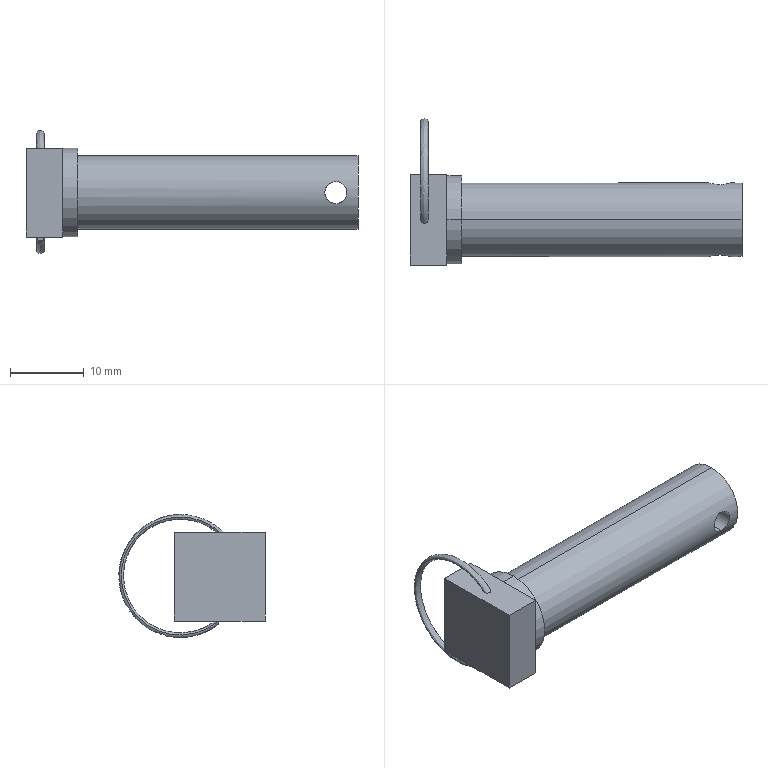Part | SolidWorks | features ICE 3, BaseBody 1, Sweep 1 | 1 solid | 20 faces | box 45 x 19.844 x 16.686 mm | volume 3901 mm3 | plane 10 | cylinder 8 | spline 2 | commonest cylinder face diameters 0.2 x2 3 x2 10 x2 12 x2
STEP:
#1=CARTESIAN_POINT('',(-3.551,0.1842,-6.026));
#2=VERTEX_POINT('',#1);
#3=CARTESIAN_POINT('',(-2.551,0.1842,-6.026));
#4=VERTEX_POINT('',#3);
#5=CARTESIAN_POINT('',(-3.051,0.1842,-6.026));
#6=DIRECTION('',(0.,-0.9908,-0.1352));
#7=DIRECTION('',(1.,0.,0.));
#8=AXIS2_PLACEMENT_3D('',#5,#6,#7);
#9=CIRCLE('',#8,0.5);
#10=EDGE_CURVE('',#2,#4,#9,.T.);
#11=ORIENTED_EDGE('',*,*,#10,.F.);
#12=CARTESIAN_POINT('',(-3.551,0.,6.026));
#13=VERTEX_POINT('',#12);
#14=CARTESIAN_POINT('',(-3.551,0.1842,-6.026));
#15=CARTESIAN_POINT('',(-3.551,6.268,-11.175));
#16=CARTESIAN_POINT('',(-3.551,13.473,-7.767));
#17=CARTESIAN_POINT('',(-3.551,13.351,0.2026));
#18=CARTESIAN_POINT('',(-3.551,13.229,8.172));
#19=CARTESIAN_POINT('',(-3.551,5.924,11.358));
#20=CARTESIAN_POINT('',(-3.551,0.,6.026));
#21=(BOUNDED_CURVE()B_SPLINE_CURVE(3,(#14,#15,#16,#17,#18,#19,#20),.UNSPECIFIED.,.F.,.F.)B_SPLINE_CURVE_WITH_KNOTS((4,3,4),(0.,0.5,1.),.UNSPECIFIED.)CURVE()GEOMETRIC_REPRESENTATION_ITEM()RATIONAL_B_SPLINE_CURVE((1.,0.6092,0.6092,1.,0.6092,0.6092,1.))REPRESENTATION_ITEM(''));
#22=EDGE_CURVE('',#2,#13,#21,.T.);
#23=ORIENTED_EDGE('',*,*,#22,.T.);
#24=CARTESIAN_POINT('',(-2.551,0.,6.026));
#25=VERTEX_POINT('',#24);
#26=CARTESIAN_POINT('',(-3.051,0.,6.026));
#27=DIRECTION('',(0.,0.,1.));
#28=DIRECTION('',(1.,0.,0.));
#29=AXIS2_PLACEMENT_3D('',#26,#27,#28);
#30=CIRCLE('',#29,0.5);
#31=EDGE_CURVE('',#13,#25,#30,.T.);
#32=ORIENTED_EDGE('',*,*,#31,.T.);
#33=CARTESIAN_POINT('',(-2.551,0.1842,-6.026));
#34=CARTESIAN_POINT('',(-2.551,6.268,-11.175));
#35=CARTESIAN_POINT('',(-2.551,13.473,-7.767));
#36=CARTESIAN_POINT('',(-2.551,13.351,0.2026));
#37=CARTESIAN_POINT('',(-2.551,13.229,8.172));
#38=CARTESIAN_POINT('',(-2.551,5.924,11.358));
#39=CARTESIAN_POINT('',(-2.551,0.,6.026));
#40=(BOUNDED_CURVE()B_SPLINE_CURVE(3,(#33,#34,#35,#36,#37,#38,#39),.UNSPECIFIED.,.F.,.T.)B_SPLINE_CURVE_WITH_KNOTS((4,3,4),(0.,0.5,1.),.UNSPECIFIED.)CURVE()GEOMETRIC_REPRESENTATION_ITEM()RATIONAL_B_SPLINE_CURVE((1.,0.6092,0.6092,1.,0.6092,0.6092,1.))REPRESENTATION_ITEM(''));
#41=EDGE_CURVE('',#4,#25,#40,.T.);
#42=ORIENTED_EDGE('',*,*,#41,.F.);
#43=EDGE_LOOP('',(#11,#23,#32,#42));
#44=FACE_OUTER_BOUND('',#43,.T.);
#45=CARTESIAN_POINT('',(-2.551,0.1842,-6.026));
#46=CARTESIAN_POINT('',(-2.551,6.268,-11.175));
#47=CARTESIAN_POINT('',(-2.551,13.473,-7.767));
#48=CARTESIAN_POINT('',(-2.551,13.351,0.2026));
#49=CARTESIAN_POINT('',(-2.551,13.229,8.172));
#50=CARTESIAN_POINT('',(-2.551,5.924,11.358));
#51=CARTESIAN_POINT('',(-2.551,0.,6.026));
#52=CARTESIAN_POINT('',(-2.551,0.04897,-5.036));
#53=CARTESIAN_POINT('',(-2.551,5.146,-10.319));
#54=CARTESIAN_POINT('',(-2.551,12.065,-7.865));
#55=CARTESIAN_POINT('',(-2.551,12.693,-0.5508));
#56=CARTESIAN_POINT('',(-2.551,13.322,6.763));
#57=CARTESIAN_POINT('',(-2.551,6.924,10.362));
#58=CARTESIAN_POINT('',(-2.551,1.,6.026));
#59=CARTESIAN_POINT('',(-3.551,0.04897,-5.036));
#60=CARTESIAN_POINT('',(-3.551,5.146,-10.319));
#61=CARTESIAN_POINT('',(-3.551,12.065,-7.865));
#62=CARTESIAN_POINT('',(-3.551,12.693,-0.5508));
#63=CARTESIAN_POINT('',(-3.551,13.322,6.763));
#64=CARTESIAN_POINT('',(-3.551,6.924,10.362));
#65=CARTESIAN_POINT('',(-3.551,1.,6.026));
#66=CARTESIAN_POINT('',(-3.551,0.1842,-6.026));
#67=CARTESIAN_POINT('',(-3.551,6.268,-11.175));
#68=CARTESIAN_POINT('',(-3.551,13.473,-7.767));
#69=CARTESIAN_POINT('',(-3.551,13.351,0.2026));
#70=CARTESIAN_POINT('',(-3.551,13.229,8.172));
#71=CARTESIAN_POINT('',(-3.551,5.924,11.358));
#72=CARTESIAN_POINT('',(-3.551,0.,6.026));
#73=CARTESIAN_POINT('',(-3.551,0.3194,-7.017));
#74=CARTESIAN_POINT('',(-3.551,7.391,-12.031));
#75=CARTESIAN_POINT('',(-3.551,14.881,-7.668));
#76=CARTESIAN_POINT('',(-3.551,14.009,0.956));
#77=CARTESIAN_POINT('',(-3.551,13.136,9.58));
#78=CARTESIAN_POINT('',(-3.551,4.924,12.355));
#79=CARTESIAN_POINT('',(-3.551,-1.,6.026));
#80=CARTESIAN_POINT('',(-2.551,0.3194,-7.017));
#81=CARTESIAN_POINT('',(-2.551,7.391,-12.031));
#82=CARTESIAN_POINT('',(-2.551,14.881,-7.668));
#83=CARTESIAN_POINT('',(-2.551,14.009,0.956));
#84=CARTESIAN_POINT('',(-2.551,13.136,9.58));
#85=CARTESIAN_POINT('',(-2.551,4.924,12.355));
#86=CARTESIAN_POINT('',(-2.551,-1.,6.026));
#87=CARTESIAN_POINT('',(-2.551,0.1842,-6.026));
#88=CARTESIAN_POINT('',(-2.551,6.268,-11.175));
#89=CARTESIAN_POINT('',(-2.551,13.473,-7.767));
#90=CARTESIAN_POINT('',(-2.551,13.351,0.2026));
#91=CARTESIAN_POINT('',(-2.551,13.229,8.172));
#92=CARTESIAN_POINT('',(-2.551,5.924,11.358));
#93=CARTESIAN_POINT('',(-2.551,0.,6.026));
#94=(BOUNDED_SURFACE()B_SPLINE_SURFACE(3,3,((#45,#46,#47,#48,#49,#50,#51),(#52,#53,#54,#55,#56,#57,#58),(#59,#60,#61,#62,#63,#64,#65),(#66,#67,#68,#69,#70,#71,#72),(#73,#74,#75,#76,#77,#78,#79),(#80,#81,#82,#83,#84,#85,#86),(#87,#88,#89,#90,#91,#92,#93)),.UNSPECIFIED.,.T.,.F.,.F.)B_SPLINE_SURFACE_WITH_KNOTS((4,3,4),(4,3,4),(0.,0.5,1.),(0.,0.5,1.),.UNSPECIFIED.)GEOMETRIC_REPRESENTATION_ITEM()RATIONAL_B_SPLINE_SURFACE(((1.,0.6092,0.6092,1.,0.6092,0.6092,1.),(0.3333,0.2031,0.2031,0.3333,0.2031,0.2031,0.3333),(0.3333,0.2031,0.2031,0.3333,0.2031,0.2031,0.3333),(1.,0.6092,0.6092,1.,0.6092,0.6092,1.),(0.3333,0.2031,0.2031,0.3333,0.2031,0.2031,0.3333),(0.3333,0.2031,0.2031,0.3333,0.2031,0.2031,0.3333),(1.,0.6092,0.6092,1.,0.6092,0.6092,1.)))REPRESENTATION_ITEM('')SURFACE());
#95=ADVANCED_FACE('',(#44),#94,.F.);
#96=CARTESIAN_POINT('',(-3.151,0.,-6.026));
#97=VERTEX_POINT('',#96);
#98=CARTESIAN_POINT('',(-2.951,0.,-6.026));
#99=VERTEX_POINT('',#98);
#100=CARTESIAN_POINT('',(-3.051,0.,-6.026));
#101=DIRECTION('',(0.,0.,1.));
#102=DIRECTION('',(1.,0.,0.));
#103=AXIS2_PLACEMENT_3D('',#100,#101,#102);
#104=CIRCLE('',#103,0.1);
#105=EDGE_CURVE('',#97,#99,#104,.T.);
#106=ORIENTED_EDGE('',*,*,#105,.F.);
#107=CARTESIAN_POINT('',(-3.151,0.,6.026));
#108=VERTEX_POINT('',#107);
#109=CARTESIAN_POINT('',(-3.151,0.,-6.026));
#110=DIRECTION('',(0.,0.,1.));
#111=VECTOR('',#110,1000.);
#112=LINE('',#109,#111);
#113=EDGE_CURVE('',#97,#108,#112,.T.);
#114=ORIENTED_EDGE('',*,*,#113,.T.);
#115=CARTESIAN_POINT('',(-2.951,0.,6.026));
#116=VERTEX_POINT('',#115);
#117=CARTESIAN_POINT('',(-3.051,0.,6.026));
#118=DIRECTION('',(0.,0.,1.));
#119=DIRECTION('',(1.,0.,0.));
#120=AXIS2_PLACEMENT_3D('',#117,#118,#119);
#121=CIRCLE('',#120,0.1);
#122=EDGE_CURVE('',#108,#116,#121,.T.);
#123=ORIENTED_EDGE('',*,*,#122,.T.);
#124=CARTESIAN_POINT('',(-2.951,0.,-6.026));
#125=DIRECTION('',(0.,0.,1.));
#126=VECTOR('',#125,1000.);
#127=LINE('',#124,#126);
#128=EDGE_CURVE('',#99,#116,#127,.T.);
#129=ORIENTED_EDGE('',*,*,#128,.F.);
#130=EDGE_LOOP('',(#106,#114,#123,#129));
#131=FACE_OUTER_BOUND('',#130,.T.);
#132=CARTESIAN_POINT('',(-3.051,0.,-6.026));
#133=DIRECTION('',(0.,0.,1.));
#134=DIRECTION('',(1.,0.,0.));
#135=AXIS2_PLACEMENT_3D('',#132,#133,#134);
#136=CYLINDRICAL_SURFACE('',#135,0.1);
#137=ADVANCED_FACE('',(#131),#136,.F.);
#138=CARTESIAN_POINT('',(37.,4.77,1.5));
#139=VERTEX_POINT('',#138);
#140=CARTESIAN_POINT('',(37.,4.77,-1.5));
#141=VERTEX_POINT('',#140);
#142=CARTESIAN_POINT('',(37.,4.77,1.5));
#143=CARTESIAN_POINT('',(36.9,4.77,1.5));
#144=CARTESIAN_POINT('',(36.802,4.773,1.49));
#145=CARTESIAN_POINT('',(36.61,4.785,1.452));
#146=CARTESIAN_POINT('',(36.514,4.794,1.423));
#147=CARTESIAN_POINT('',(36.333,4.815,1.347));
#148=CARTESIAN_POINT('',(36.247,4.828,1.301));
#149=CARTESIAN_POINT('',(36.085,4.856,1.192));
#150=CARTESIAN_POINT('',(36.008,4.871,1.129));
#151=CARTESIAN_POINT('',(35.802,4.916,0.9233));
#152=CARTESIAN_POINT('',(35.69,4.946,0.7569));
#153=CARTESIAN_POINT('',(35.54,4.988,0.3965));
#154=CARTESIAN_POINT('',(35.5,5.,0.1984));
#155=CARTESIAN_POINT('',(35.5,5.,-0.09698));
#156=CARTESIAN_POINT('',(35.51,4.997,-0.197));
#157=CARTESIAN_POINT('',(35.548,4.986,-0.3898));
#158=CARTESIAN_POINT('',(35.577,4.977,-0.4837));
#159=CARTESIAN_POINT('',(35.69,4.946,-0.7572));
#160=CARTESIAN_POINT('',(35.801,4.916,-0.9219));
#161=CARTESIAN_POINT('',(36.008,4.871,-1.13));
#162=CARTESIAN_POINT('',(36.083,4.856,-1.191));
#163=CARTESIAN_POINT('',(36.245,4.828,-1.3));
#164=CARTESIAN_POINT('',(36.333,4.815,-1.347));
#165=CARTESIAN_POINT('',(36.604,4.783,-1.46));
#166=CARTESIAN_POINT('',(36.801,4.77,-1.5));
#167=CARTESIAN_POINT('',(37.,4.77,-1.5));
#168=B_SPLINE_CURVE_WITH_KNOTS('',3,(#142,#143,#144,#145,#146,#147,#148,#149,#150,#151,#152,#153,#154,#155,#156,#157,#158,#159,#160,#161,#162,#163,#164,#165,#166,#167),.UNSPECIFIED.,.F.,.F.,(4,2,2,2,2,2,2,2,2,2,2,2,4),(0.004715,0.00501,0.005305,0.005599,0.005894,0.006483,0.007073,0.007367,0.007662,0.008251,0.008546,0.008841,0.00943),.UNSPECIFIED.);
#169=EDGE_CURVE('',#139,#141,#168,.T.);
#170=ORIENTED_EDGE('',*,*,#169,.T.);
#171=CARTESIAN_POINT('',(37.,4.77,-1.5));
#172=CARTESIAN_POINT('',(37.1,4.77,-1.5));
#173=CARTESIAN_POINT('',(37.198,4.773,-1.49));
#174=CARTESIAN_POINT('',(37.39,4.785,-1.452));
#175=CARTESIAN_POINT('',(37.486,4.794,-1.423));
#176=CARTESIAN_POINT('',(37.667,4.815,-1.347));
#177=CARTESIAN_POINT('',(37.753,4.828,-1.301));
#178=CARTESIAN_POINT('',(37.915,4.856,-1.192));
#179=CARTESIAN_POINT('',(37.992,4.871,-1.129));
#180=CARTESIAN_POINT('',(38.198,4.916,-0.9233));
#181=CARTESIAN_POINT('',(38.31,4.946,-0.7569));
#182=CARTESIAN_POINT('',(38.46,4.988,-0.3965));
#183=CARTESIAN_POINT('',(38.5,5.,-0.1984));
#184=CARTESIAN_POINT('',(38.5,5.,0.09698));
#185=CARTESIAN_POINT('',(38.49,4.997,0.197));
#186=CARTESIAN_POINT('',(38.452,4.986,0.3898));
#187=CARTESIAN_POINT('',(38.423,4.977,0.4837));
#188=CARTESIAN_POINT('',(38.31,4.946,0.7572));
#189=CARTESIAN_POINT('',(38.199,4.916,0.9219));
#190=CARTESIAN_POINT('',(37.992,4.871,1.13));
#191=CARTESIAN_POINT('',(37.917,4.856,1.191));
#192=CARTESIAN_POINT('',(37.755,4.828,1.3));
#193=CARTESIAN_POINT('',(37.667,4.815,1.347));
#194=CARTESIAN_POINT('',(37.396,4.783,1.46));
#195=CARTESIAN_POINT('',(37.199,4.77,1.5));
#196=CARTESIAN_POINT('',(37.,4.77,1.5));
#197=B_SPLINE_CURVE_WITH_KNOTS('',3,(#171,#172,#173,#174,#175,#176,#177,#178,#179,#180,#181,#182,#183,#184,#185,#186,#187,#188,#189,#190,#191,#192,#193,#194,#195,#196),.UNSPECIFIED.,.F.,.F.,(4,2,2,2,2,2,2,2,2,2,2,2,4),(0.,0.0002947,0.0005894,0.0008841,0.001179,0.001768,0.002358,0.002652,0.002947,0.003536,0.003831,0.004126,0.004715),.UNSPECIFIED.);
#198=EDGE_CURVE('',#141,#139,#197,.T.);
#199=ORIENTED_EDGE('',*,*,#198,.T.);
#200=EDGE_LOOP('',(#170,#199));
#201=FACE_BOUND('',#200,.T.);
#202=CARTESIAN_POINT('',(2.,0.,-5.));
#203=VERTEX_POINT('',#202);
#204=CARTESIAN_POINT('',(2.,0.,5.));
#205=VERTEX_POINT('',#204);
#206=CARTESIAN_POINT('',(2.,0.,0.));
#207=DIRECTION('',(1.,0.,0.));
#208=DIRECTION('',(0.,0.,-1.));
#209=AXIS2_PLACEMENT_3D('',#206,#207,#208);
#210=CIRCLE('',#209,5.);
#211=EDGE_CURVE('',#203,#205,#210,.T.);
#212=ORIENTED_EDGE('',*,*,#211,.T.);
#213=CARTESIAN_POINT('',(40.,0.,5.));
#214=VERTEX_POINT('',#213);
#215=CARTESIAN_POINT('',(0.,0.,5.));
#216=DIRECTION('',(1.,0.,0.));
#217=VECTOR('',#216,1000.);
#218=LINE('',#215,#217);
#219=EDGE_CURVE('',#205,#214,#218,.T.);
#220=ORIENTED_EDGE('',*,*,#219,.T.);
#221=CARTESIAN_POINT('',(40.,0.,-5.));
#222=VERTEX_POINT('',#221);
#223=CARTESIAN_POINT('',(40.,0.,0.));
#224=DIRECTION('',(-1.,0.,0.));
#225=DIRECTION('',(0.,0.,-1.));
#226=AXIS2_PLACEMENT_3D('',#223,#224,#225);
#227=CIRCLE('',#226,5.);
#228=EDGE_CURVE('',#214,#222,#227,.T.);
#229=ORIENTED_EDGE('',*,*,#228,.T.);
#230=CARTESIAN_POINT('',(0.,0.,-5.));
#231=DIRECTION('',(1.,0.,0.));
#232=VECTOR('',#231,1000.);
#233=LINE('',#230,#232);
#234=EDGE_CURVE('',#203,#222,#233,.T.);
#235=ORIENTED_EDGE('',*,*,#234,.F.);
#236=EDGE_LOOP('',(#212,#220,#229,#235));
#237=FACE_OUTER_BOUND('',#236,.T.);
#238=CARTESIAN_POINT('',(0.,0.,0.));
#239=DIRECTION('',(1.,0.,0.));
#240=DIRECTION('',(0.,0.,-1.));
#241=AXIS2_PLACEMENT_3D('',#238,#239,#240);
#242=CYLINDRICAL_SURFACE('',#241,5.);
#243=ADVANCED_FACE('',(#201,#237),#242,.T.);
#244=CARTESIAN_POINT('',(37.,-4.77,-1.5));
#245=VERTEX_POINT('',#244);
#246=CARTESIAN_POINT('',(37.,-4.77,1.5));
#247=VERTEX_POINT('',#246);
#248=CARTESIAN_POINT('',(37.,-4.77,-1.5));
#249=CARTESIAN_POINT('',(36.9,-4.77,-1.5));
#250=CARTESIAN_POINT('',(36.802,-4.773,-1.49));
#251=CARTESIAN_POINT('',(36.61,-4.785,-1.452));
#252=CARTESIAN_POINT('',(36.514,-4.794,-1.423));
#253=CARTESIAN_POINT('',(36.333,-4.815,-1.347));
#254=CARTESIAN_POINT('',(36.247,-4.828,-1.301));
#255=CARTESIAN_POINT('',(36.085,-4.856,-1.192));
#256=CARTESIAN_POINT('',(36.008,-4.871,-1.129));
#257=CARTESIAN_POINT('',(35.802,-4.916,-0.9233));
#258=CARTESIAN_POINT('',(35.69,-4.946,-0.7569));
#259=CARTESIAN_POINT('',(35.54,-4.988,-0.3965));
#260=CARTESIAN_POINT('',(35.5,-5.,-0.1984));
#261=CARTESIAN_POINT('',(35.5,-5.,0.09698));
#262=CARTESIAN_POINT('',(35.51,-4.997,0.197));
#263=CARTESIAN_POINT('',(35.548,-4.986,0.3898));
#264=CARTESIAN_POINT('',(35.577,-4.977,0.4837));
#265=CARTESIAN_POINT('',(35.69,-4.946,0.7572));
#266=CARTESIAN_POINT('',(35.801,-4.916,0.9219));
#267=CARTESIAN_POINT('',(36.008,-4.871,1.13));
#268=CARTESIAN_POINT('',(36.083,-4.856,1.191));
#269=CARTESIAN_POINT('',(36.245,-4.828,1.3));
#270=CARTESIAN_POINT('',(36.333,-4.815,1.347));
#271=CARTESIAN_POINT('',(36.604,-4.783,1.46));
#272=CARTESIAN_POINT('',(36.801,-4.77,1.5));
#273=CARTESIAN_POINT('',(37.,-4.77,1.5));
#274=B_SPLINE_CURVE_WITH_KNOTS('',3,(#248,#249,#250,#251,#252,#253,#254,#255,#256,#257,#258,#259,#260,#261,#262,#263,#264,#265,#266,#267,#268,#269,#270,#271,#272,#273),.UNSPECIFIED.,.F.,.F.,(4,2,2,2,2,2,2,2,2,2,2,2,4),(0.,0.0002947,0.0005894,0.0008841,0.001179,0.001768,0.002358,0.002652,0.002947,0.003536,0.003831,0.004126,0.004715),.UNSPECIFIED.);
#275=EDGE_CURVE('',#245,#247,#274,.T.);
#276=ORIENTED_EDGE('',*,*,#275,.F.);
#277=CARTESIAN_POINT('',(37.,-6.,-1.5));
#278=DIRECTION('',(0.,1.,0.));
#279=VECTOR('',#278,1000.);
#280=LINE('',#277,#279);
#281=EDGE_CURVE('',#245,#141,#280,.T.);
#282=ORIENTED_EDGE('',*,*,#281,.T.);
#283=ORIENTED_EDGE('',*,*,#169,.F.);
#284=CARTESIAN_POINT('',(37.,-6.,1.5));
#285=DIRECTION('',(0.,1.,0.));
#286=VECTOR('',#285,1000.);
#287=LINE('',#284,#286);
#288=EDGE_CURVE('',#247,#139,#287,.T.);
#289=ORIENTED_EDGE('',*,*,#288,.F.);
#290=EDGE_LOOP('',(#276,#282,#283,#289));
#291=FACE_OUTER_BOUND('',#290,.T.);
#292=CARTESIAN_POINT('',(37.,-6.,0.));
#293=DIRECTION('',(0.,1.,0.));
#294=DIRECTION('',(0.,0.,1.));
#295=AXIS2_PLACEMENT_3D('',#292,#293,#294);
#296=CYLINDRICAL_SURFACE('',#295,1.5);
#297=ADVANCED_FACE('',(#291),#296,.F.);
#298=CARTESIAN_POINT('',(0.,0.,-6.));
#299=VERTEX_POINT('',#298);
#300=CARTESIAN_POINT('',(0.,0.,6.));
#301=VERTEX_POINT('',#300);
#302=CARTESIAN_POINT('',(0.,0.,0.));
#303=DIRECTION('',(1.,0.,0.));
#304=DIRECTION('',(0.,0.,-1.));
#305=AXIS2_PLACEMENT_3D('',#302,#303,#304);
#306=CIRCLE('',#305,6.);
#307=EDGE_CURVE('',#299,#301,#306,.T.);
#308=ORIENTED_EDGE('',*,*,#307,.T.);
#309=CARTESIAN_POINT('',(2.,0.,6.));
#310=VERTEX_POINT('',#309);
#311=CARTESIAN_POINT('',(0.,0.,6.));
#312=DIRECTION('',(1.,0.,0.));
#313=VECTOR('',#312,1000.);
#314=LINE('',#311,#313);
#315=EDGE_CURVE('',#301,#310,#314,.T.);
#316=ORIENTED_EDGE('',*,*,#315,.T.);
#317=CARTESIAN_POINT('',(2.,0.,-6.));
#318=VERTEX_POINT('',#317);
#319=CARTESIAN_POINT('',(2.,0.,0.));
#320=DIRECTION('',(1.,0.,0.));
#321=DIRECTION('',(0.,0.,-1.));
#322=AXIS2_PLACEMENT_3D('',#319,#320,#321);
#323=CIRCLE('',#322,6.);
#324=EDGE_CURVE('',#318,#310,#323,.T.);
#325=ORIENTED_EDGE('',*,*,#324,.F.);
#326=CARTESIAN_POINT('',(0.,0.,-6.));
#327=DIRECTION('',(1.,0.,0.));
#328=VECTOR('',#327,1000.);
#329=LINE('',#326,#328);
#330=EDGE_CURVE('',#299,#318,#329,.T.);
#331=ORIENTED_EDGE('',*,*,#330,.F.);
#332=EDGE_LOOP('',(#308,#316,#325,#331));
#333=FACE_OUTER_BOUND('',#332,.T.);
#334=CARTESIAN_POINT('',(0.,0.,0.));
#335=DIRECTION('',(1.,0.,0.));
#336=DIRECTION('',(0.,0.,-1.));
#337=AXIS2_PLACEMENT_3D('',#334,#335,#336);
#338=CYLINDRICAL_SURFACE('',#337,6.);
#339=ADVANCED_FACE('',(#333),#338,.T.);
#340=ORIENTED_EDGE('',*,*,#219,.F.);
#341=CARTESIAN_POINT('',(2.,0.,0.));
#342=DIRECTION('',(1.,0.,0.));
#343=DIRECTION('',(0.,0.,-1.));
#344=AXIS2_PLACEMENT_3D('',#341,#342,#343);
#345=CIRCLE('',#344,5.);
#346=EDGE_CURVE('',#205,#203,#345,.T.);
#347=ORIENTED_EDGE('',*,*,#346,.T.);
#348=ORIENTED_EDGE('',*,*,#234,.T.);
#349=CARTESIAN_POINT('',(40.,0.,0.));
#350=DIRECTION('',(-1.,0.,0.));
#351=DIRECTION('',(0.,0.,-1.));
#352=AXIS2_PLACEMENT_3D('',#349,#350,#351);
#353=CIRCLE('',#352,5.);
#354=EDGE_CURVE('',#222,#214,#353,.T.);
#355=ORIENTED_EDGE('',*,*,#354,.T.);
#356=EDGE_LOOP('',(#340,#347,#348,#355));
#357=FACE_OUTER_BOUND('',#356,.T.);
#358=CARTESIAN_POINT('',(37.,-4.77,1.5));
#359=CARTESIAN_POINT('',(37.1,-4.77,1.5));
#360=CARTESIAN_POINT('',(37.198,-4.773,1.49));
#361=CARTESIAN_POINT('',(37.39,-4.785,1.452));
#362=CARTESIAN_POINT('',(37.486,-4.794,1.423));
#363=CARTESIAN_POINT('',(37.667,-4.815,1.347));
#364=CARTESIAN_POINT('',(37.753,-4.828,1.301));
#365=CARTESIAN_POINT('',(37.915,-4.856,1.192));
#366=CARTESIAN_POINT('',(37.992,-4.871,1.129));
#367=CARTESIAN_POINT('',(38.198,-4.916,0.9233));
#368=CARTESIAN_POINT('',(38.31,-4.946,0.7569));
#369=CARTESIAN_POINT('',(38.46,-4.988,0.3965));
#370=CARTESIAN_POINT('',(38.5,-5.,0.1984));
#371=CARTESIAN_POINT('',(38.5,-5.,-0.09698));
#372=CARTESIAN_POINT('',(38.49,-4.997,-0.197));
#373=CARTESIAN_POINT('',(38.452,-4.986,-0.3898));
#374=CARTESIAN_POINT('',(38.423,-4.977,-0.4837));
#375=CARTESIAN_POINT('',(38.31,-4.946,-0.7572));
#376=CARTESIAN_POINT('',(38.199,-4.916,-0.9219));
#377=CARTESIAN_POINT('',(37.992,-4.871,-1.13));
#378=CARTESIAN_POINT('',(37.917,-4.856,-1.191));
#379=CARTESIAN_POINT('',(37.755,-4.828,-1.3));
#380=CARTESIAN_POINT('',(37.667,-4.815,-1.347));
#381=CARTESIAN_POINT('',(37.396,-4.783,-1.46));
#382=CARTESIAN_POINT('',(37.199,-4.77,-1.5));
#383=CARTESIAN_POINT('',(37.,-4.77,-1.5));
#384=B_SPLINE_CURVE_WITH_KNOTS('',3,(#358,#359,#360,#361,#362,#363,#364,#365,#366,#367,#368,#369,#370,#371,#372,#373,#374,#375,#376,#377,#378,#379,#380,#381,#382,#383),.UNSPECIFIED.,.F.,.F.,(4,2,2,2,2,2,2,2,2,2,2,2,4),(0.004715,0.00501,0.005305,0.005599,0.005894,0.006483,0.007073,0.007367,0.007662,0.008251,0.008546,0.008841,0.00943),.UNSPECIFIED.);
#385=EDGE_CURVE('',#247,#245,#384,.T.);
#386=ORIENTED_EDGE('',*,*,#385,.T.);
#387=ORIENTED_EDGE('',*,*,#275,.T.);
#388=EDGE_LOOP('',(#386,#387));
#389=FACE_BOUND('',#388,.T.);
#390=CARTESIAN_POINT('',(0.,0.,0.));
#391=DIRECTION('',(1.,0.,0.));
#392=DIRECTION('',(0.,0.,-1.));
#393=AXIS2_PLACEMENT_3D('',#390,#391,#392);
#394=CYLINDRICAL_SURFACE('',#393,5.);
#395=ADVANCED_FACE('',(#357,#389),#394,.T.);
#396=ORIENTED_EDGE('',*,*,#281,.F.);
#397=ORIENTED_EDGE('',*,*,#385,.F.);
#398=ORIENTED_EDGE('',*,*,#288,.T.);
#399=ORIENTED_EDGE('',*,*,#198,.F.);
#400=EDGE_LOOP('',(#396,#397,#398,#399));
#401=FACE_OUTER_BOUND('',#400,.T.);
#402=CARTESIAN_POINT('',(37.,-6.,0.));
#403=DIRECTION('',(0.,1.,0.));
#404=DIRECTION('',(0.,0.,1.));
#405=AXIS2_PLACEMENT_3D('',#402,#403,#404);
#406=CYLINDRICAL_SURFACE('',#405,1.5);
#407=ADVANCED_FACE('',(#401),#406,.F.);
#408=ORIENTED_EDGE('',*,*,#354,.F.);
#409=ORIENTED_EDGE('',*,*,#228,.F.);
#410=EDGE_LOOP('',(#408,#409));
#411=FACE_OUTER_BOUND('',#410,.T.);
#412=CARTESIAN_POINT('',(40.,5.,0.));
#413=DIRECTION('',(1.,0.,0.));
#414=DIRECTION('',(0.,0.,-1.));
#415=AXIS2_PLACEMENT_3D('',#412,#413,#414);
#416=PLANE('',#415);
#417=ADVANCED_FACE('',(#411),#416,.T.);
#418=ORIENTED_EDGE('',*,*,#211,.F.);
#419=ORIENTED_EDGE('',*,*,#346,.F.);
#420=EDGE_LOOP('',(#418,#419));
#421=FACE_BOUND('',#420,.T.);
#422=ORIENTED_EDGE('',*,*,#324,.T.);
#423=CARTESIAN_POINT('',(2.,0.,0.));
#424=DIRECTION('',(1.,0.,0.));
#425=DIRECTION('',(0.,0.,-1.));
#426=AXIS2_PLACEMENT_3D('',#423,#424,#425);
#427=CIRCLE('',#426,6.);
#428=EDGE_CURVE('',#310,#318,#427,.T.);
#429=ORIENTED_EDGE('',*,*,#428,.T.);
#430=EDGE_LOOP('',(#422,#429));
#431=FACE_OUTER_BOUND('',#430,.T.);
#432=CARTESIAN_POINT('',(2.,6.,0.));
#433=DIRECTION('',(1.,0.,0.));
#434=DIRECTION('',(0.,0.,-1.));
#435=AXIS2_PLACEMENT_3D('',#432,#433,#434);
#436=PLANE('',#435);
#437=ADVANCED_FACE('',(#421,#431),#436,.T.);
#438=ORIENTED_EDGE('',*,*,#315,.F.);
#439=CARTESIAN_POINT('',(0.,0.,0.));
#440=DIRECTION('',(1.,0.,0.));
#441=DIRECTION('',(0.,0.,-1.));
#442=AXIS2_PLACEMENT_3D('',#439,#440,#441);
#443=CIRCLE('',#442,6.);
#444=EDGE_CURVE('',#301,#299,#443,.T.);
#445=ORIENTED_EDGE('',*,*,#444,.T.);
#446=ORIENTED_EDGE('',*,*,#330,.T.);
#447=ORIENTED_EDGE('',*,*,#428,.F.);
#448=EDGE_LOOP('',(#438,#445,#446,#447));
#449=FACE_OUTER_BOUND('',#448,.T.);
#450=CARTESIAN_POINT('',(0.,0.,0.));
#451=DIRECTION('',(1.,0.,0.));
#452=DIRECTION('',(0.,0.,-1.));
#453=AXIS2_PLACEMENT_3D('',#450,#451,#452);
#454=CYLINDRICAL_SURFACE('',#453,6.);
#455=ADVANCED_FACE('',(#449),#454,.T.);
#456=CARTESIAN_POINT('',(-3.051,0.,6.026));
#457=DIRECTION('',(0.,0.,1.));
#458=DIRECTION('',(1.,0.,0.));
#459=AXIS2_PLACEMENT_3D('',#456,#457,#458);
#460=CIRCLE('',#459,0.5);
#461=EDGE_CURVE('',#25,#13,#460,.T.);
#462=ORIENTED_EDGE('',*,*,#461,.F.);
#463=ORIENTED_EDGE('',*,*,#31,.F.);
#464=EDGE_LOOP('',(#462,#463));
#465=FACE_BOUND('',#464,.T.);
#466=CARTESIAN_POINT('',(0.,-6.15,6.026));
#467=VERTEX_POINT('',#466);
#468=CARTESIAN_POINT('',(0.,6.15,6.026));
#469=VERTEX_POINT('',#468);
#470=CARTESIAN_POINT('',(0.,6.15,6.026));
#471=DIRECTION('',(0.,1.,0.));
#472=VECTOR('',#471,1000.);
#473=LINE('',#470,#472);
#474=EDGE_CURVE('',#467,#469,#473,.T.);
#475=ORIENTED_EDGE('',*,*,#474,.T.);
#476=CARTESIAN_POINT('',(-5.,6.15,6.026));
#477=VERTEX_POINT('',#476);
#478=CARTESIAN_POINT('',(-5.,6.15,6.026));
#479=DIRECTION('',(1.,0.,0.));
#480=VECTOR('',#479,1000.);
#481=LINE('',#478,#480);
#482=EDGE_CURVE('',#477,#469,#481,.T.);
#483=ORIENTED_EDGE('',*,*,#482,.F.);
#484=CARTESIAN_POINT('',(-5.,-6.15,6.026));
#485=VERTEX_POINT('',#484);
#486=CARTESIAN_POINT('',(-5.,6.15,6.026));
#487=DIRECTION('',(0.,1.,0.));
#488=VECTOR('',#487,1000.);
#489=LINE('',#486,#488);
#490=EDGE_CURVE('',#485,#477,#489,.T.);
#491=ORIENTED_EDGE('',*,*,#490,.F.);
#492=CARTESIAN_POINT('',(-5.,-6.15,6.026));
#493=DIRECTION('',(1.,0.,0.));
#494=VECTOR('',#493,1000.);
#495=LINE('',#492,#494);
#496=EDGE_CURVE('',#485,#467,#495,.T.);
#497=ORIENTED_EDGE('',*,*,#496,.T.);
#498=EDGE_LOOP('',(#475,#483,#491,#497));
#499=FACE_OUTER_BOUND('',#498,.T.);
#500=CARTESIAN_POINT('',(-5.,6.15,6.026));
#501=DIRECTION('',(0.,0.,-1.));
#502=DIRECTION('',(-1.,0.,0.));
#503=AXIS2_PLACEMENT_3D('',#500,#501,#502);
#504=PLANE('',#503);
#505=ADVANCED_FACE('',(#465,#499),#504,.F.);
#506=CARTESIAN_POINT('',(0.,6.15,-6.026));
#507=VERTEX_POINT('',#506);
#508=CARTESIAN_POINT('',(0.,6.15,-6.026));
#509=DIRECTION('',(0.,0.,-1.));
#510=VECTOR('',#509,1000.);
#511=LINE('',#508,#510);
#512=EDGE_CURVE('',#469,#507,#511,.T.);
#513=ORIENTED_EDGE('',*,*,#512,.T.);
#514=CARTESIAN_POINT('',(-5.,6.15,-6.026));
#515=VERTEX_POINT('',#514);
#516=CARTESIAN_POINT('',(-5.,6.15,-6.026));
#517=DIRECTION('',(1.,0.,0.));
#518=VECTOR('',#517,1000.);
#519=LINE('',#516,#518);
#520=EDGE_CURVE('',#515,#507,#519,.T.);
#521=ORIENTED_EDGE('',*,*,#520,.F.);
#522=CARTESIAN_POINT('',(-5.,6.15,-6.026));
#523=DIRECTION('',(0.,0.,-1.));
#524=VECTOR('',#523,1000.);
#525=LINE('',#522,#524);
#526=EDGE_CURVE('',#477,#515,#525,.T.);
#527=ORIENTED_EDGE('',*,*,#526,.F.);
#528=ORIENTED_EDGE('',*,*,#482,.T.);
#529=EDGE_LOOP('',(#513,#521,#527,#528));
#530=FACE_OUTER_BOUND('',#529,.T.);
#531=CARTESIAN_POINT('',(-5.,6.15,-6.026));
#532=DIRECTION('',(0.,-1.,0.));
#533=DIRECTION('',(0.,0.,-1.));
#534=AXIS2_PLACEMENT_3D('',#531,#532,#533);
#535=PLANE('',#534);
#536=ADVANCED_FACE('',(#530),#535,.F.);
#537=CARTESIAN_POINT('',(-3.551,0.1842,-6.026));
#538=CARTESIAN_POINT('',(-3.551,0.3188,-6.026));
#539=CARTESIAN_POINT('',(-3.499,0.4508,-6.026));
#540=CARTESIAN_POINT('',(-3.316,0.6448,-6.026));
#541=CARTESIAN_POINT('',(-3.184,0.7038,-6.026));
#542=CARTESIAN_POINT('',(-2.918,0.7041,-6.026));
#543=CARTESIAN_POINT('',(-2.787,0.6462,-6.026));
#544=CARTESIAN_POINT('',(-2.602,0.4504,-6.026));
#545=CARTESIAN_POINT('',(-2.551,0.3188,-6.026));
#546=CARTESIAN_POINT('',(-2.551,0.1842,-6.026));
#547=B_SPLINE_CURVE_WITH_KNOTS('',3,(#537,#538,#539,#540,#541,#542,#543,#544,#545,#546),.UNSPECIFIED.,.F.,.F.,(4,2,2,2,4),(0.,0.0003982,0.0007963,0.001194,0.001593),.UNSPECIFIED.);
#548=EDGE_CURVE('',#2,#4,#547,.T.);
#549=ORIENTED_EDGE('',*,*,#548,.F.);
#550=CARTESIAN_POINT('',(-5.,0.1842,-6.026));
#551=DIRECTION('',(1.,0.,0.));
#552=VECTOR('',#551,1000.);
#553=LINE('',#550,#552);
#554=EDGE_CURVE('',#2,#4,#553,.T.);
#555=ORIENTED_EDGE('',*,*,#554,.T.);
#556=EDGE_LOOP('',(#549,#555));
#557=FACE_BOUND('',#556,.T.);
#558=CARTESIAN_POINT('',(-3.051,0.,-6.026));
#559=DIRECTION('',(0.,0.,1.));
#560=DIRECTION('',(1.,0.,0.));
#561=AXIS2_PLACEMENT_3D('',#558,#559,#560);
#562=CIRCLE('',#561,0.1);
#563=EDGE_CURVE('',#99,#97,#562,.T.);
#564=ORIENTED_EDGE('',*,*,#563,.T.);
#565=ORIENTED_EDGE('',*,*,#105,.T.);
#566=EDGE_LOOP('',(#564,#565));
#567=FACE_BOUND('',#566,.T.);
#568=CARTESIAN_POINT('',(0.,-6.15,-6.026));
#569=VERTEX_POINT('',#568);
#570=CARTESIAN_POINT('',(0.,6.15,-6.026));
#571=DIRECTION('',(0.,-1.,0.));
#572=VECTOR('',#571,1000.);
#573=LINE('',#570,#572);
#574=EDGE_CURVE('',#507,#569,#573,.T.);
#575=ORIENTED_EDGE('',*,*,#574,.T.);
#576=CARTESIAN_POINT('',(-5.,-6.15,-6.026));
#577=VERTEX_POINT('',#576);
#578=CARTESIAN_POINT('',(-5.,-6.15,-6.026));
#579=DIRECTION('',(1.,0.,0.));
#580=VECTOR('',#579,1000.);
#581=LINE('',#578,#580);
#582=EDGE_CURVE('',#577,#569,#581,.T.);
#583=ORIENTED_EDGE('',*,*,#582,.F.);
#584=CARTESIAN_POINT('',(-5.,6.15,-6.026));
#585=DIRECTION('',(0.,-1.,0.));
#586=VECTOR('',#585,1000.);
#587=LINE('',#584,#586);
#588=EDGE_CURVE('',#515,#577,#587,.T.);
#589=ORIENTED_EDGE('',*,*,#588,.F.);
#590=ORIENTED_EDGE('',*,*,#520,.T.);
#591=EDGE_LOOP('',(#575,#583,#589,#590));
#592=FACE_OUTER_BOUND('',#591,.T.);
#593=CARTESIAN_POINT('',(-5.,6.15,-6.026));
#594=DIRECTION('',(0.,0.,1.));
#595=DIRECTION('',(1.,0.,0.));
#596=AXIS2_PLACEMENT_3D('',#593,#594,#595);
#597=PLANE('',#596);
#598=ADVANCED_FACE('',(#557,#567,#592),#597,.F.);
#599=CARTESIAN_POINT('',(0.,-6.15,-6.026));
#600=DIRECTION('',(0.,0.,1.));
#601=VECTOR('',#600,1000.);
#602=LINE('',#599,#601);
#603=EDGE_CURVE('',#569,#467,#602,.T.);
#604=ORIENTED_EDGE('',*,*,#603,.T.);
#605=ORIENTED_EDGE('',*,*,#496,.F.);
#606=CARTESIAN_POINT('',(-5.,-6.15,-6.026));
#607=DIRECTION('',(0.,0.,1.));
#608=VECTOR('',#607,1000.);
#609=LINE('',#606,#608);
#610=EDGE_CURVE('',#577,#485,#609,.T.);
#611=ORIENTED_EDGE('',*,*,#610,.F.);
#612=ORIENTED_EDGE('',*,*,#582,.T.);
#613=EDGE_LOOP('',(#604,#605,#611,#612));
#614=FACE_OUTER_BOUND('',#613,.T.);
#615=CARTESIAN_POINT('',(-5.,-6.15,-6.026));
#616=DIRECTION('',(0.,1.,0.));
#617=DIRECTION('',(0.,0.,1.));
#618=AXIS2_PLACEMENT_3D('',#615,#616,#617);
#619=PLANE('',#618);
#620=ADVANCED_FACE('',(#614),#619,.F.);
#621=ORIENTED_EDGE('',*,*,#490,.T.);
#622=ORIENTED_EDGE('',*,*,#526,.T.);
#623=ORIENTED_EDGE('',*,*,#588,.T.);
#624=ORIENTED_EDGE('',*,*,#610,.T.);
#625=EDGE_LOOP('',(#621,#622,#623,#624));
#626=FACE_OUTER_BOUND('',#625,.T.);
#627=CARTESIAN_POINT('',(-5.,0.,0.));
#628=DIRECTION('',(-1.,0.,0.));
#629=DIRECTION('',(0.,0.,1.));
#630=AXIS2_PLACEMENT_3D('',#627,#628,#629);
#631=PLANE('',#630);
#632=ADVANCED_FACE('',(#626),#631,.T.);
#633=ORIENTED_EDGE('',*,*,#307,.F.);
#634=ORIENTED_EDGE('',*,*,#444,.F.);
#635=EDGE_LOOP('',(#633,#634));
#636=FACE_BOUND('',#635,.T.);
#637=ORIENTED_EDGE('',*,*,#474,.F.);
#638=ORIENTED_EDGE('',*,*,#603,.F.);
#639=ORIENTED_EDGE('',*,*,#574,.F.);
#640=ORIENTED_EDGE('',*,*,#512,.F.);
#641=EDGE_LOOP('',(#637,#638,#639,#640));
#642=FACE_OUTER_BOUND('',#641,.T.);
#643=CARTESIAN_POINT('',(0.,0.,0.));
#644=DIRECTION('',(-1.,0.,0.));
#645=DIRECTION('',(0.,0.,1.));
#646=AXIS2_PLACEMENT_3D('',#643,#644,#645);
#647=PLANE('',#646);
#648=ADVANCED_FACE('',(#636,#642),#647,.F.);
#649=ORIENTED_EDGE('',*,*,#113,.F.);
#650=ORIENTED_EDGE('',*,*,#563,.F.);
#651=ORIENTED_EDGE('',*,*,#128,.T.);
#652=CARTESIAN_POINT('',(-3.051,0.,6.026));
#653=DIRECTION('',(0.,0.,1.));
#654=DIRECTION('',(1.,0.,0.));
#655=AXIS2_PLACEMENT_3D('',#652,#653,#654);
#656=CIRCLE('',#655,0.1);
#657=EDGE_CURVE('',#116,#108,#656,.T.);
#658=ORIENTED_EDGE('',*,*,#657,.T.);
#659=EDGE_LOOP('',(#649,#650,#651,#658));
#660=FACE_OUTER_BOUND('',#659,.T.);
#661=CARTESIAN_POINT('',(-3.051,0.,-6.026));
#662=DIRECTION('',(0.,0.,1.));
#663=DIRECTION('',(1.,0.,0.));
#664=AXIS2_PLACEMENT_3D('',#661,#662,#663);
#665=CYLINDRICAL_SURFACE('',#664,0.1);
#666=ADVANCED_FACE('',(#660),#665,.F.);
#667=ORIENTED_EDGE('',*,*,#22,.F.);
#668=ORIENTED_EDGE('',*,*,#548,.T.);
#669=ORIENTED_EDGE('',*,*,#41,.T.);
#670=ORIENTED_EDGE('',*,*,#461,.T.);
#671=EDGE_LOOP('',(#667,#668,#669,#670));
#672=FACE_OUTER_BOUND('',#671,.T.);
#673=CARTESIAN_POINT('',(-2.551,0.1842,-6.026));
#674=CARTESIAN_POINT('',(-2.551,6.268,-11.175));
#675=CARTESIAN_POINT('',(-2.551,13.473,-7.767));
#676=CARTESIAN_POINT('',(-2.551,13.351,0.2026));
#677=CARTESIAN_POINT('',(-2.551,13.229,8.172));
#678=CARTESIAN_POINT('',(-2.551,5.924,11.358));
#679=CARTESIAN_POINT('',(-2.551,0.,6.026));
#680=CARTESIAN_POINT('',(-2.551,0.04897,-5.036));
#681=CARTESIAN_POINT('',(-2.551,5.146,-10.319));
#682=CARTESIAN_POINT('',(-2.551,12.065,-7.865));
#683=CARTESIAN_POINT('',(-2.551,12.693,-0.5508));
#684=CARTESIAN_POINT('',(-2.551,13.322,6.763));
#685=CARTESIAN_POINT('',(-2.551,6.924,10.362));
#686=CARTESIAN_POINT('',(-2.551,1.,6.026));
#687=CARTESIAN_POINT('',(-3.551,0.04897,-5.036));
#688=CARTESIAN_POINT('',(-3.551,5.146,-10.319));
#689=CARTESIAN_POINT('',(-3.551,12.065,-7.865));
#690=CARTESIAN_POINT('',(-3.551,12.693,-0.5508));
#691=CARTESIAN_POINT('',(-3.551,13.322,6.763));
#692=CARTESIAN_POINT('',(-3.551,6.924,10.362));
#693=CARTESIAN_POINT('',(-3.551,1.,6.026));
#694=CARTESIAN_POINT('',(-3.551,0.1842,-6.026));
#695=CARTESIAN_POINT('',(-3.551,6.268,-11.175));
#696=CARTESIAN_POINT('',(-3.551,13.473,-7.767));
#697=CARTESIAN_POINT('',(-3.551,13.351,0.2026));
#698=CARTESIAN_POINT('',(-3.551,13.229,8.172));
#699=CARTESIAN_POINT('',(-3.551,5.924,11.358));
#700=CARTESIAN_POINT('',(-3.551,0.,6.026));
#701=CARTESIAN_POINT('',(-3.551,0.3194,-7.017));
#702=CARTESIAN_POINT('',(-3.551,7.391,-12.031));
#703=CARTESIAN_POINT('',(-3.551,14.881,-7.668));
#704=CARTESIAN_POINT('',(-3.551,14.009,0.956));
#705=CARTESIAN_POINT('',(-3.551,13.136,9.58));
#706=CARTESIAN_POINT('',(-3.551,4.924,12.355));
#707=CARTESIAN_POINT('',(-3.551,-1.,6.026));
#708=CARTESIAN_POINT('',(-2.551,0.3194,-7.017));
#709=CARTESIAN_POINT('',(-2.551,7.391,-12.031));
#710=CARTESIAN_POINT('',(-2.551,14.881,-7.668));
#711=CARTESIAN_POINT('',(-2.551,14.009,0.956));
#712=CARTESIAN_POINT('',(-2.551,13.136,9.58));
#713=CARTESIAN_POINT('',(-2.551,4.924,12.355));
#714=CARTESIAN_POINT('',(-2.551,-1.,6.026));
#715=CARTESIAN_POINT('',(-2.551,0.1842,-6.026));
#716=CARTESIAN_POINT('',(-2.551,6.268,-11.175));
#717=CARTESIAN_POINT('',(-2.551,13.473,-7.767));
#718=CARTESIAN_POINT('',(-2.551,13.351,0.2026));
#719=CARTESIAN_POINT('',(-2.551,13.229,8.172));
#720=CARTESIAN_POINT('',(-2.551,5.924,11.358));
#721=CARTESIAN_POINT('',(-2.551,0.,6.026));
#722=(BOUNDED_SURFACE()B_SPLINE_SURFACE(3,3,((#673,#674,#675,#676,#677,#678,#679),(#680,#681,#682,#683,#684,#685,#686),(#687,#688,#689,#690,#691,#692,#693),(#694,#695,#696,#697,#698,#699,#700),(#701,#702,#703,#704,#705,#706,#707),(#708,#709,#710,#711,#712,#713,#714),(#715,#716,#717,#718,#719,#720,#721)),.UNSPECIFIED.,.T.,.F.,.F.)B_SPLINE_SURFACE_WITH_KNOTS((4,3,4),(4,3,4),(0.,0.5,1.),(0.,0.5,1.),.UNSPECIFIED.)GEOMETRIC_REPRESENTATION_ITEM()RATIONAL_B_SPLINE_SURFACE(((1.,0.6092,0.6092,1.,0.6092,0.6092,1.),(0.3333,0.2031,0.2031,0.3333,0.2031,0.2031,0.3333),(0.3333,0.2031,0.2031,0.3333,0.2031,0.2031,0.3333),(1.,0.6092,0.6092,1.,0.6092,0.6092,1.),(0.3333,0.2031,0.2031,0.3333,0.2031,0.2031,0.3333),(0.3333,0.2031,0.2031,0.3333,0.2031,0.2031,0.3333),(1.,0.6092,0.6092,1.,0.6092,0.6092,1.)))REPRESENTATION_ITEM('')SURFACE());
#723=ADVANCED_FACE('',(#672),#722,.F.);
#724=ORIENTED_EDGE('',*,*,#554,.F.);
#725=ORIENTED_EDGE('',*,*,#10,.T.);
#726=EDGE_LOOP('',(#724,#725));
#727=FACE_OUTER_BOUND('',#726,.T.);
#728=CARTESIAN_POINT('',(-3.051,0.1842,-6.026));
#729=DIRECTION('',(0.,-0.9908,-0.1352));
#730=DIRECTION('',(1.,0.,0.));
#731=AXIS2_PLACEMENT_3D('',#728,#729,#730);
#732=PLANE('',#731);
#733=ADVANCED_FACE('',(#727),#732,.T.);
#734=ORIENTED_EDGE('',*,*,#657,.F.);
#735=ORIENTED_EDGE('',*,*,#122,.F.);
#736=EDGE_LOOP('',(#734,#735));
#737=FACE_OUTER_BOUND('',#736,.T.);
#738=CARTESIAN_POINT('',(-3.051,0.,6.026));
#739=DIRECTION('',(0.,0.,1.));
#740=DIRECTION('',(1.,0.,0.));
#741=AXIS2_PLACEMENT_3D('',#738,#739,#740);
#742=PLANE('',#741);
#743=ADVANCED_FACE('',(#737),#742,.F.);
#744=CLOSED_SHELL('',(#95,#137,#243,#297,#339,#395,#407,#417,#437,#455,#505,#536,#598,#620,#632,#648,#666,#723,#733,#743));
#745=MANIFOLD_SOLID_BREP('',#744);
#746=CARTESIAN_POINT('',(0.,0.,0.));
#747=DIRECTION('',(0.,0.,1.));
#748=DIRECTION('',(1.,0.,0.));
#749=AXIS2_PLACEMENT_3D('',#746,#747,#748);
#750=(LENGTH_UNIT()NAMED_UNIT(*)SI_UNIT(.MILLI.,.METRE.));
#751=UNCERTAINTY_MEASURE_WITH_UNIT(LENGTH_MEASURE(0.00001),#750,'','');
#752=(NAMED_UNIT(*)PLANE_ANGLE_UNIT()SI_UNIT($,.RADIAN.));
#753=(NAMED_UNIT(*)SI_UNIT($,.STERADIAN.)SOLID_ANGLE_UNIT());
#754=(GEOMETRIC_REPRESENTATION_CONTEXT(3)GLOBAL_UNCERTAINTY_ASSIGNED_CONTEXT((#751))GLOBAL_UNIT_ASSIGNED_CONTEXT((#750,#752,#753))REPRESENTATION_CONTEXT('',''));
#755=ADVANCED_BREP_SHAPE_REPRESENTATION('',(#745,#749),#754);